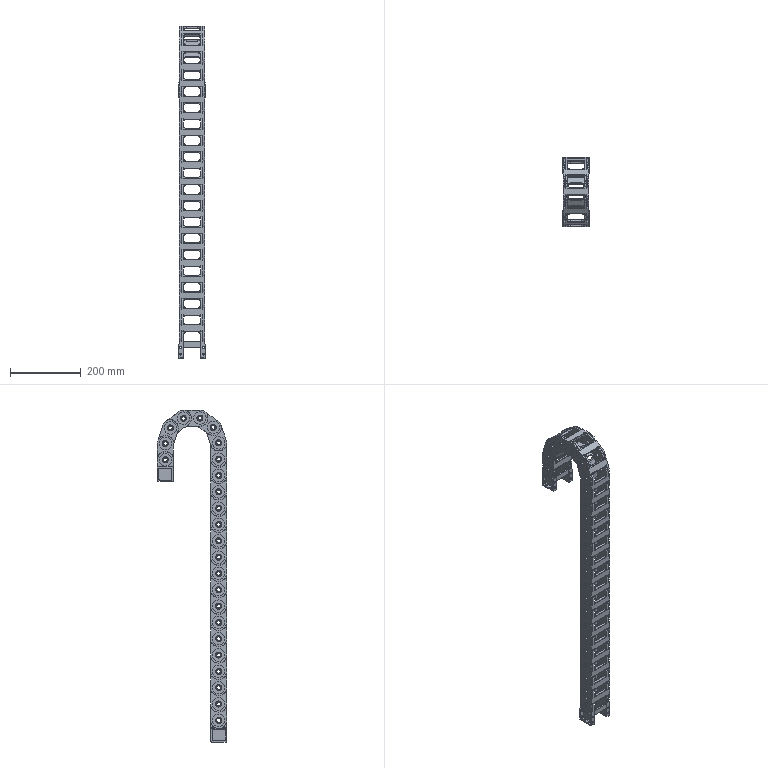Part | SolidWorks | features ReferencePattern 9, LocalLPattern 1 | 25 solids | 6380 faces | volume 1169113 mm3 | cylinder 3988 | plane 2392 | commonest cylinder face diameters 2 x680 1 x460 4 x288 20.12 x240 41.64 x230 17.1 x192